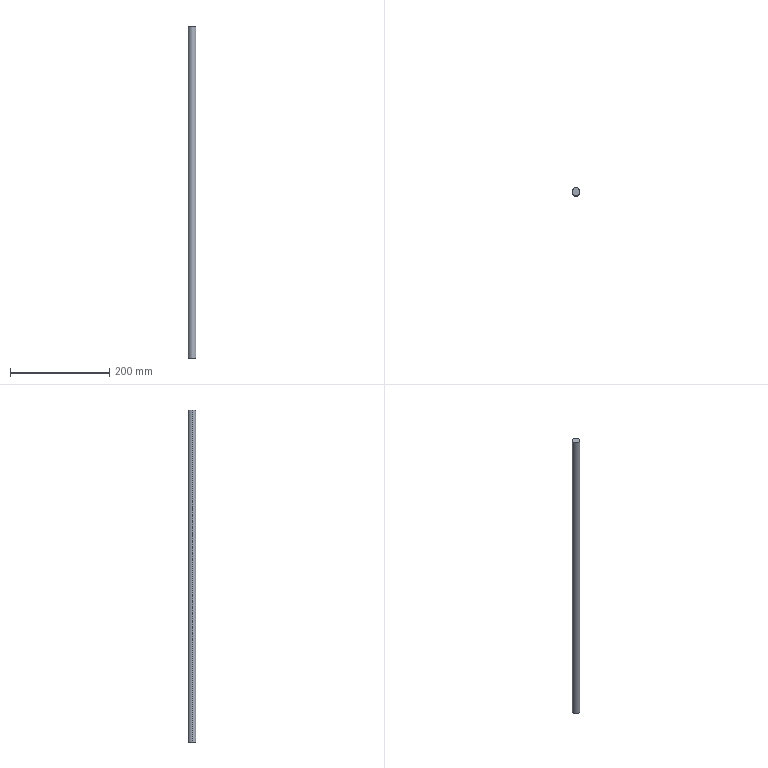Part | SolidWorks | features Extrusion 1 | 1 solid | 4 faces | box 16 x 16 x 669 mm | volume 134510 mm3 | cylinder 2 | plane 2 | commonest cylinder face diameters 16 x2
STEP:
#1=CARTESIAN_POINT('',(8.,0.,669.));
#2=VERTEX_POINT('',#1);
#3=CARTESIAN_POINT('',(-8.,0.,669.));
#4=VERTEX_POINT('',#3);
#5=CARTESIAN_POINT('',(0.,0.,669.));
#6=DIRECTION('',(0.,0.,1.));
#7=DIRECTION('',(1.,0.,0.));
#8=AXIS2_PLACEMENT_3D('',#5,#6,#7);
#9=CIRCLE('',#8,8.);
#10=EDGE_CURVE('',#2,#4,#9,.T.);
#11=ORIENTED_EDGE('',*,*,#10,.F.);
#12=CARTESIAN_POINT('',(8.,0.,0.));
#13=VERTEX_POINT('',#12);
#14=CARTESIAN_POINT('',(8.,0.,669.));
#15=DIRECTION('',(0.,0.,-1.));
#16=VECTOR('',#15,1000.);
#17=LINE('',#14,#16);
#18=EDGE_CURVE('',#2,#13,#17,.T.);
#19=ORIENTED_EDGE('',*,*,#18,.T.);
#20=CARTESIAN_POINT('',(-8.,0.,0.));
#21=VERTEX_POINT('',#20);
#22=CARTESIAN_POINT('',(0.,0.,0.));
#23=DIRECTION('',(0.,0.,1.));
#24=DIRECTION('',(1.,0.,0.));
#25=AXIS2_PLACEMENT_3D('',#22,#23,#24);
#26=CIRCLE('',#25,8.);
#27=EDGE_CURVE('',#13,#21,#26,.T.);
#28=ORIENTED_EDGE('',*,*,#27,.T.);
#29=CARTESIAN_POINT('',(-8.,0.,669.));
#30=DIRECTION('',(0.,0.,-1.));
#31=VECTOR('',#30,1000.);
#32=LINE('',#29,#31);
#33=EDGE_CURVE('',#4,#21,#32,.T.);
#34=ORIENTED_EDGE('',*,*,#33,.F.);
#35=EDGE_LOOP('',(#11,#19,#28,#34));
#36=FACE_OUTER_BOUND('',#35,.T.);
#37=CARTESIAN_POINT('',(0.,0.,669.));
#38=DIRECTION('',(0.,0.,-1.));
#39=DIRECTION('',(-1.,0.,0.));
#40=AXIS2_PLACEMENT_3D('',#37,#38,#39);
#41=CYLINDRICAL_SURFACE('',#40,8.);
#42=ADVANCED_FACE('',(#36),#41,.T.);
#43=ORIENTED_EDGE('',*,*,#18,.F.);
#44=CARTESIAN_POINT('',(0.,0.,669.));
#45=DIRECTION('',(0.,0.,1.));
#46=DIRECTION('',(1.,0.,0.));
#47=AXIS2_PLACEMENT_3D('',#44,#45,#46);
#48=CIRCLE('',#47,8.);
#49=EDGE_CURVE('',#4,#2,#48,.T.);
#50=ORIENTED_EDGE('',*,*,#49,.F.);
#51=ORIENTED_EDGE('',*,*,#33,.T.);
#52=CARTESIAN_POINT('',(0.,0.,0.));
#53=DIRECTION('',(0.,0.,1.));
#54=DIRECTION('',(1.,0.,0.));
#55=AXIS2_PLACEMENT_3D('',#52,#53,#54);
#56=CIRCLE('',#55,8.);
#57=EDGE_CURVE('',#21,#13,#56,.T.);
#58=ORIENTED_EDGE('',*,*,#57,.T.);
#59=EDGE_LOOP('',(#43,#50,#51,#58));
#60=FACE_OUTER_BOUND('',#59,.T.);
#61=CARTESIAN_POINT('',(0.,0.,669.));
#62=DIRECTION('',(0.,0.,-1.));
#63=DIRECTION('',(-1.,0.,0.));
#64=AXIS2_PLACEMENT_3D('',#61,#62,#63);
#65=CYLINDRICAL_SURFACE('',#64,8.);
#66=ADVANCED_FACE('',(#60),#65,.T.);
#67=ORIENTED_EDGE('',*,*,#49,.T.);
#68=ORIENTED_EDGE('',*,*,#10,.T.);
#69=EDGE_LOOP('',(#67,#68));
#70=FACE_OUTER_BOUND('',#69,.T.);
#71=CARTESIAN_POINT('',(0.,0.,669.));
#72=DIRECTION('',(0.,0.,1.));
#73=DIRECTION('',(1.,0.,0.));
#74=AXIS2_PLACEMENT_3D('',#71,#72,#73);
#75=PLANE('',#74);
#76=ADVANCED_FACE('',(#70),#75,.T.);
#77=ORIENTED_EDGE('',*,*,#57,.F.);
#78=ORIENTED_EDGE('',*,*,#27,.F.);
#79=EDGE_LOOP('',(#77,#78));
#80=FACE_OUTER_BOUND('',#79,.T.);
#81=CARTESIAN_POINT('',(0.,0.,0.));
#82=DIRECTION('',(0.,0.,1.));
#83=DIRECTION('',(1.,0.,0.));
#84=AXIS2_PLACEMENT_3D('',#81,#82,#83);
#85=PLANE('',#84);
#86=ADVANCED_FACE('',(#80),#85,.F.);
#87=CLOSED_SHELL('',(#42,#66,#76,#86));
#88=MANIFOLD_SOLID_BREP('',#87);
#89=CARTESIAN_POINT('',(0.,0.,0.));
#90=DIRECTION('',(0.,0.,1.));
#91=DIRECTION('',(1.,0.,0.));
#92=AXIS2_PLACEMENT_3D('',#89,#90,#91);
#93=(LENGTH_UNIT()NAMED_UNIT(*)SI_UNIT(.MILLI.,.METRE.));
#94=UNCERTAINTY_MEASURE_WITH_UNIT(LENGTH_MEASURE(0.00001),#93,'','');
#95=(NAMED_UNIT(*)PLANE_ANGLE_UNIT()SI_UNIT($,.RADIAN.));
#96=(NAMED_UNIT(*)SI_UNIT($,.STERADIAN.)SOLID_ANGLE_UNIT());
#97=(GEOMETRIC_REPRESENTATION_CONTEXT(3)GLOBAL_UNCERTAINTY_ASSIGNED_CONTEXT((#94))GLOBAL_UNIT_ASSIGNED_CONTEXT((#93,#95,#96))REPRESENTATION_CONTEXT('',''));
#98=ADVANCED_BREP_SHAPE_REPRESENTATION('',(#88,#92),#97);